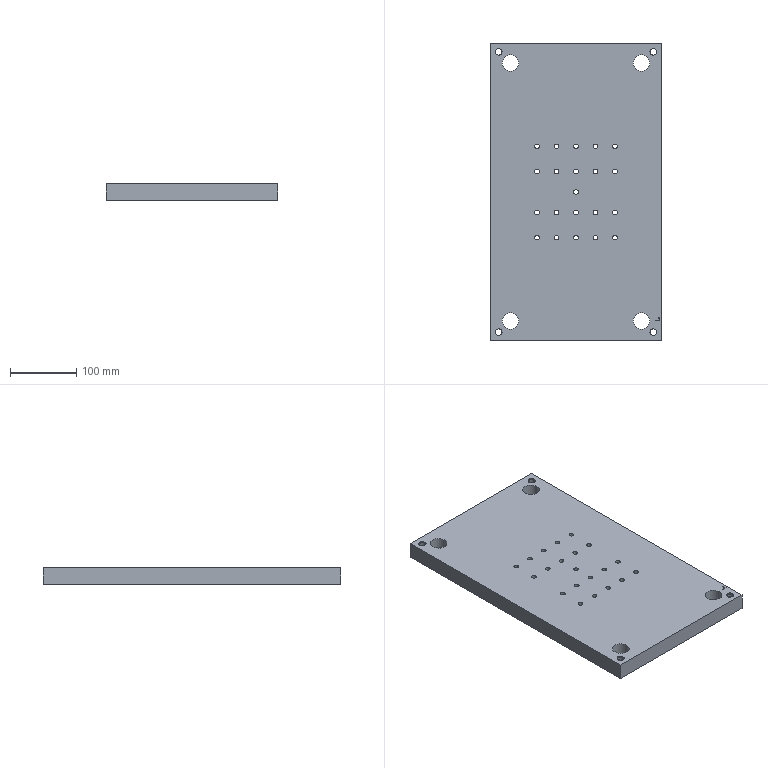Part | NX | features solid 2 | 1 solid | 116 faces | box 260 x 450 x 25 mm | volume 2831486 mm3 | cylinder 62 | plane 54 | commonest cylinder face diameters 7 x21 11 x21 10.2 x4 11.7 x4 12 x4 25 x4